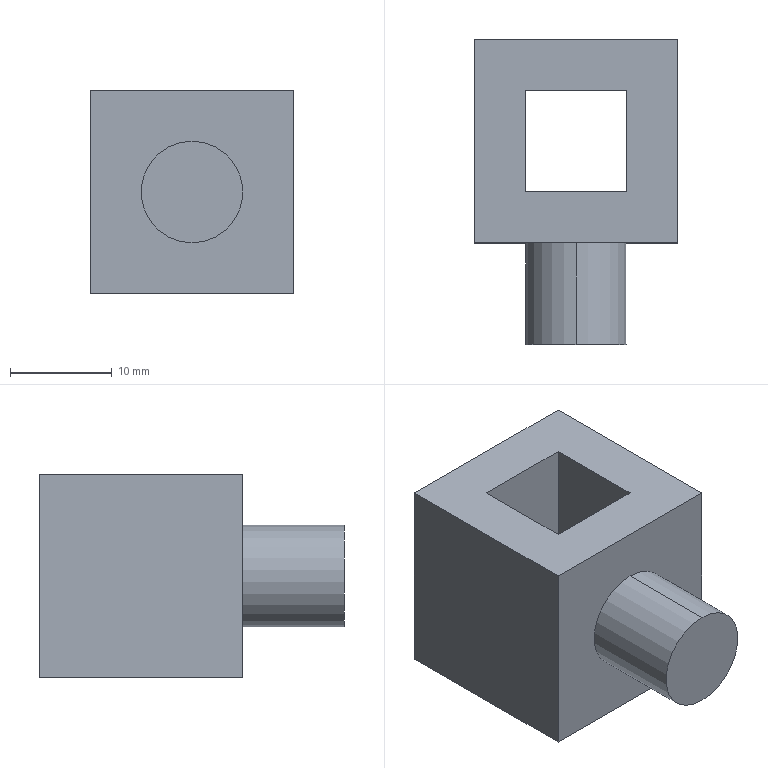Part | SolidWorks | features Extrusion 1, ICE 1 | 1 solid | 13 faces | box 20 x 30 x 20 mm | volume 6785 mm3 | plane 11 | cylinder 2 | commonest cylinder face diameters 10 x2
STEP:
#1=CARTESIAN_POINT('',(5.,-15.,-5.));
#2=VERTEX_POINT('',#1);
#3=CARTESIAN_POINT('',(5.,-15.,5.));
#4=VERTEX_POINT('',#3);
#5=CARTESIAN_POINT('',(5.,-15.,0.));
#6=DIRECTION('',(0.,-1.,0.));
#7=DIRECTION('',(0.,0.,-1.));
#8=AXIS2_PLACEMENT_3D('',#5,#6,#7);
#9=CIRCLE('',#8,5.);
#10=EDGE_CURVE('',#2,#4,#9,.T.);
#11=ORIENTED_EDGE('',*,*,#10,.F.);
#12=CARTESIAN_POINT('',(5.,-5.,-5.));
#13=VERTEX_POINT('',#12);
#14=CARTESIAN_POINT('',(5.,-15.,-5.));
#15=DIRECTION('',(0.,1.,0.));
#16=VECTOR('',#15,1000.);
#17=LINE('',#14,#16);
#18=EDGE_CURVE('',#2,#13,#17,.T.);
#19=ORIENTED_EDGE('',*,*,#18,.T.);
#20=CARTESIAN_POINT('',(5.,-5.,5.));
#21=VERTEX_POINT('',#20);
#22=CARTESIAN_POINT('',(5.,-5.,0.));
#23=DIRECTION('',(0.,-1.,0.));
#24=DIRECTION('',(0.,0.,1.));
#25=AXIS2_PLACEMENT_3D('',#22,#23,#24);
#26=CIRCLE('',#25,5.);
#27=EDGE_CURVE('',#13,#21,#26,.T.);
#28=ORIENTED_EDGE('',*,*,#27,.T.);
#29=CARTESIAN_POINT('',(5.,-15.,5.));
#30=DIRECTION('',(0.,1.,0.));
#31=VECTOR('',#30,1000.);
#32=LINE('',#29,#31);
#33=EDGE_CURVE('',#4,#21,#32,.T.);
#34=ORIENTED_EDGE('',*,*,#33,.F.);
#35=EDGE_LOOP('',(#11,#19,#28,#34));
#36=FACE_OUTER_BOUND('',#35,.T.);
#37=CARTESIAN_POINT('',(5.,-15.,0.));
#38=DIRECTION('',(0.,1.,0.));
#39=DIRECTION('',(0.,0.,1.));
#40=AXIS2_PLACEMENT_3D('',#37,#38,#39);
#41=CYLINDRICAL_SURFACE('',#40,5.);
#42=ADVANCED_FACE('',(#36),#41,.T.);
#43=CARTESIAN_POINT('',(-5.,-5.,-10.));
#44=VERTEX_POINT('',#43);
#45=CARTESIAN_POINT('',(15.,-5.,-10.));
#46=VERTEX_POINT('',#45);
#47=CARTESIAN_POINT('',(-5.,-5.,-10.));
#48=DIRECTION('',(1.,0.,0.));
#49=VECTOR('',#48,1000.);
#50=LINE('',#47,#49);
#51=EDGE_CURVE('',#44,#46,#50,.T.);
#52=ORIENTED_EDGE('',*,*,#51,.T.);
#53=CARTESIAN_POINT('',(15.,-5.,10.));
#54=VERTEX_POINT('',#53);
#55=CARTESIAN_POINT('',(15.,-5.,10.));
#56=DIRECTION('',(0.,0.,-1.));
#57=VECTOR('',#56,1000.);
#58=LINE('',#55,#57);
#59=EDGE_CURVE('',#54,#46,#58,.T.);
#60=ORIENTED_EDGE('',*,*,#59,.F.);
#61=CARTESIAN_POINT('',(-5.,-5.,10.));
#62=VERTEX_POINT('',#61);
#63=CARTESIAN_POINT('',(-5.,-5.,10.));
#64=DIRECTION('',(1.,0.,0.));
#65=VECTOR('',#64,1000.);
#66=LINE('',#63,#65);
#67=EDGE_CURVE('',#62,#54,#66,.T.);
#68=ORIENTED_EDGE('',*,*,#67,.F.);
#69=CARTESIAN_POINT('',(-5.,-5.,10.));
#70=DIRECTION('',(0.,0.,-1.));
#71=VECTOR('',#70,1000.);
#72=LINE('',#69,#71);
#73=EDGE_CURVE('',#62,#44,#72,.T.);
#74=ORIENTED_EDGE('',*,*,#73,.T.);
#75=EDGE_LOOP('',(#52,#60,#68,#74));
#76=FACE_OUTER_BOUND('',#75,.T.);
#77=CARTESIAN_POINT('',(5.,-5.,0.));
#78=DIRECTION('',(0.,-1.,0.));
#79=DIRECTION('',(0.,0.,1.));
#80=AXIS2_PLACEMENT_3D('',#77,#78,#79);
#81=CIRCLE('',#80,5.);
#82=EDGE_CURVE('',#21,#13,#81,.T.);
#83=ORIENTED_EDGE('',*,*,#82,.F.);
#84=ORIENTED_EDGE('',*,*,#27,.F.);
#85=EDGE_LOOP('',(#83,#84));
#86=FACE_BOUND('',#85,.T.);
#87=CARTESIAN_POINT('',(-5.,-5.,10.));
#88=DIRECTION('',(0.,1.,0.));
#89=DIRECTION('',(0.,0.,1.));
#90=AXIS2_PLACEMENT_3D('',#87,#88,#89);
#91=PLANE('',#90);
#92=ADVANCED_FACE('',(#76,#86),#91,.F.);
#93=CARTESIAN_POINT('',(-5.,15.,10.));
#94=VERTEX_POINT('',#93);
#95=CARTESIAN_POINT('',(-5.,-5.,10.));
#96=DIRECTION('',(0.,-1.,0.));
#97=VECTOR('',#96,1000.);
#98=LINE('',#95,#97);
#99=EDGE_CURVE('',#94,#62,#98,.T.);
#100=ORIENTED_EDGE('',*,*,#99,.T.);
#101=ORIENTED_EDGE('',*,*,#67,.T.);
#102=CARTESIAN_POINT('',(15.,15.,10.));
#103=VERTEX_POINT('',#102);
#104=CARTESIAN_POINT('',(15.,-5.,10.));
#105=DIRECTION('',(0.,1.,0.));
#106=VECTOR('',#105,1000.);
#107=LINE('',#104,#106);
#108=EDGE_CURVE('',#54,#103,#107,.T.);
#109=ORIENTED_EDGE('',*,*,#108,.T.);
#110=CARTESIAN_POINT('',(-5.,15.,10.));
#111=DIRECTION('',(-1.,0.,0.));
#112=VECTOR('',#111,1000.);
#113=LINE('',#110,#112);
#114=EDGE_CURVE('',#103,#94,#113,.T.);
#115=ORIENTED_EDGE('',*,*,#114,.T.);
#116=EDGE_LOOP('',(#100,#101,#109,#115));
#117=FACE_OUTER_BOUND('',#116,.T.);
#118=CARTESIAN_POINT('',(0.,10.,10.));
#119=VERTEX_POINT('',#118);
#120=CARTESIAN_POINT('',(0.,0.,10.));
#121=VERTEX_POINT('',#120);
#122=CARTESIAN_POINT('',(0.,0.,10.));
#123=DIRECTION('',(0.,-1.,0.));
#124=VECTOR('',#123,1000.);
#125=LINE('',#122,#124);
#126=EDGE_CURVE('',#119,#121,#125,.T.);
#127=ORIENTED_EDGE('',*,*,#126,.F.);
#128=CARTESIAN_POINT('',(10.,10.,10.));
#129=VERTEX_POINT('',#128);
#130=CARTESIAN_POINT('',(0.,10.,10.));
#131=DIRECTION('',(-1.,0.,0.));
#132=VECTOR('',#131,1000.);
#133=LINE('',#130,#132);
#134=EDGE_CURVE('',#129,#119,#133,.T.);
#135=ORIENTED_EDGE('',*,*,#134,.F.);
#136=CARTESIAN_POINT('',(10.,0.,10.));
#137=VERTEX_POINT('',#136);
#138=CARTESIAN_POINT('',(10.,0.,10.));
#139=DIRECTION('',(0.,1.,0.));
#140=VECTOR('',#139,1000.);
#141=LINE('',#138,#140);
#142=EDGE_CURVE('',#137,#129,#141,.T.);
#143=ORIENTED_EDGE('',*,*,#142,.F.);
#144=CARTESIAN_POINT('',(0.,0.,10.));
#145=DIRECTION('',(1.,0.,0.));
#146=VECTOR('',#145,1000.);
#147=LINE('',#144,#146);
#148=EDGE_CURVE('',#121,#137,#147,.T.);
#149=ORIENTED_EDGE('',*,*,#148,.F.);
#150=EDGE_LOOP('',(#127,#135,#143,#149));
#151=FACE_BOUND('',#150,.T.);
#152=CARTESIAN_POINT('',(0.,0.,10.));
#153=DIRECTION('',(0.,0.,-1.));
#154=DIRECTION('',(-1.,0.,0.));
#155=AXIS2_PLACEMENT_3D('',#152,#153,#154);
#156=PLANE('',#155);
#157=ADVANCED_FACE('',(#117,#151),#156,.F.);
#158=CARTESIAN_POINT('',(-5.,15.,-10.));
#159=VERTEX_POINT('',#158);
#160=CARTESIAN_POINT('',(-5.,-5.,-10.));
#161=DIRECTION('',(0.,-1.,0.));
#162=VECTOR('',#161,1000.);
#163=LINE('',#160,#162);
#164=EDGE_CURVE('',#159,#44,#163,.T.);
#165=ORIENTED_EDGE('',*,*,#164,.F.);
#166=CARTESIAN_POINT('',(15.,15.,-10.));
#167=VERTEX_POINT('',#166);
#168=CARTESIAN_POINT('',(-5.,15.,-10.));
#169=DIRECTION('',(-1.,0.,0.));
#170=VECTOR('',#169,1000.);
#171=LINE('',#168,#170);
#172=EDGE_CURVE('',#167,#159,#171,.T.);
#173=ORIENTED_EDGE('',*,*,#172,.F.);
#174=CARTESIAN_POINT('',(15.,-5.,-10.));
#175=DIRECTION('',(0.,1.,0.));
#176=VECTOR('',#175,1000.);
#177=LINE('',#174,#176);
#178=EDGE_CURVE('',#46,#167,#177,.T.);
#179=ORIENTED_EDGE('',*,*,#178,.F.);
#180=ORIENTED_EDGE('',*,*,#51,.F.);
#181=EDGE_LOOP('',(#165,#173,#179,#180));
#182=FACE_OUTER_BOUND('',#181,.T.);
#183=CARTESIAN_POINT('',(10.,10.,-10.));
#184=VERTEX_POINT('',#183);
#185=CARTESIAN_POINT('',(0.,10.,-10.));
#186=VERTEX_POINT('',#185);
#187=CARTESIAN_POINT('',(0.,10.,-10.));
#188=DIRECTION('',(-1.,0.,0.));
#189=VECTOR('',#188,1000.);
#190=LINE('',#187,#189);
#191=EDGE_CURVE('',#184,#186,#190,.T.);
#192=ORIENTED_EDGE('',*,*,#191,.T.);
#193=CARTESIAN_POINT('',(0.,0.,-10.));
#194=VERTEX_POINT('',#193);
#195=CARTESIAN_POINT('',(0.,0.,-10.));
#196=DIRECTION('',(0.,-1.,0.));
#197=VECTOR('',#196,1000.);
#198=LINE('',#195,#197);
#199=EDGE_CURVE('',#186,#194,#198,.T.);
#200=ORIENTED_EDGE('',*,*,#199,.T.);
#201=CARTESIAN_POINT('',(10.,0.,-10.));
#202=VERTEX_POINT('',#201);
#203=CARTESIAN_POINT('',(0.,0.,-10.));
#204=DIRECTION('',(1.,0.,0.));
#205=VECTOR('',#204,1000.);
#206=LINE('',#203,#205);
#207=EDGE_CURVE('',#194,#202,#206,.T.);
#208=ORIENTED_EDGE('',*,*,#207,.T.);
#209=CARTESIAN_POINT('',(10.,0.,-10.));
#210=DIRECTION('',(0.,1.,0.));
#211=VECTOR('',#210,1000.);
#212=LINE('',#209,#211);
#213=EDGE_CURVE('',#202,#184,#212,.T.);
#214=ORIENTED_EDGE('',*,*,#213,.T.);
#215=EDGE_LOOP('',(#192,#200,#208,#214));
#216=FACE_BOUND('',#215,.T.);
#217=CARTESIAN_POINT('',(0.,0.,-10.));
#218=DIRECTION('',(0.,0.,-1.));
#219=DIRECTION('',(-1.,0.,0.));
#220=AXIS2_PLACEMENT_3D('',#217,#218,#219);
#221=PLANE('',#220);
#222=ADVANCED_FACE('',(#182,#216),#221,.T.);
#223=ORIENTED_EDGE('',*,*,#164,.T.);
#224=ORIENTED_EDGE('',*,*,#73,.F.);
#225=ORIENTED_EDGE('',*,*,#99,.F.);
#226=CARTESIAN_POINT('',(-5.,15.,10.));
#227=DIRECTION('',(0.,0.,-1.));
#228=VECTOR('',#227,1000.);
#229=LINE('',#226,#228);
#230=EDGE_CURVE('',#94,#159,#229,.T.);
#231=ORIENTED_EDGE('',*,*,#230,.T.);
#232=EDGE_LOOP('',(#223,#224,#225,#231));
#233=FACE_OUTER_BOUND('',#232,.T.);
#234=CARTESIAN_POINT('',(-5.,-5.,10.));
#235=DIRECTION('',(1.,0.,0.));
#236=DIRECTION('',(0.,0.,-1.));
#237=AXIS2_PLACEMENT_3D('',#234,#235,#236);
#238=PLANE('',#237);
#239=ADVANCED_FACE('',(#233),#238,.F.);
#240=ORIENTED_EDGE('',*,*,#178,.T.);
#241=CARTESIAN_POINT('',(15.,15.,10.));
#242=DIRECTION('',(0.,0.,-1.));
#243=VECTOR('',#242,1000.);
#244=LINE('',#241,#243);
#245=EDGE_CURVE('',#103,#167,#244,.T.);
#246=ORIENTED_EDGE('',*,*,#245,.F.);
#247=ORIENTED_EDGE('',*,*,#108,.F.);
#248=ORIENTED_EDGE('',*,*,#59,.T.);
#249=EDGE_LOOP('',(#240,#246,#247,#248));
#250=FACE_OUTER_BOUND('',#249,.T.);
#251=CARTESIAN_POINT('',(15.,-5.,10.));
#252=DIRECTION('',(-1.,0.,0.));
#253=DIRECTION('',(0.,0.,1.));
#254=AXIS2_PLACEMENT_3D('',#251,#252,#253);
#255=PLANE('',#254);
#256=ADVANCED_FACE('',(#250),#255,.F.);
#257=ORIENTED_EDGE('',*,*,#172,.T.);
#258=ORIENTED_EDGE('',*,*,#230,.F.);
#259=ORIENTED_EDGE('',*,*,#114,.F.);
#260=ORIENTED_EDGE('',*,*,#245,.T.);
#261=EDGE_LOOP('',(#257,#258,#259,#260));
#262=FACE_OUTER_BOUND('',#261,.T.);
#263=CARTESIAN_POINT('',(-5.,15.,10.));
#264=DIRECTION('',(0.,-1.,0.));
#265=DIRECTION('',(0.,0.,-1.));
#266=AXIS2_PLACEMENT_3D('',#263,#264,#265);
#267=PLANE('',#266);
#268=ADVANCED_FACE('',(#262),#267,.F.);
#269=ORIENTED_EDGE('',*,*,#199,.F.);
#270=CARTESIAN_POINT('',(0.,10.,10.));
#271=DIRECTION('',(0.,0.,-1.));
#272=VECTOR('',#271,1000.);
#273=LINE('',#270,#272);
#274=EDGE_CURVE('',#119,#186,#273,.T.);
#275=ORIENTED_EDGE('',*,*,#274,.F.);
#276=ORIENTED_EDGE('',*,*,#126,.T.);
#277=CARTESIAN_POINT('',(0.,0.,10.));
#278=DIRECTION('',(0.,0.,-1.));
#279=VECTOR('',#278,1000.);
#280=LINE('',#277,#279);
#281=EDGE_CURVE('',#121,#194,#280,.T.);
#282=ORIENTED_EDGE('',*,*,#281,.T.);
#283=EDGE_LOOP('',(#269,#275,#276,#282));
#284=FACE_OUTER_BOUND('',#283,.T.);
#285=CARTESIAN_POINT('',(0.,0.,10.));
#286=DIRECTION('',(1.,0.,0.));
#287=DIRECTION('',(0.,0.,-1.));
#288=AXIS2_PLACEMENT_3D('',#285,#286,#287);
#289=PLANE('',#288);
#290=ADVANCED_FACE('',(#284),#289,.T.);
#291=ORIENTED_EDGE('',*,*,#207,.F.);
#292=ORIENTED_EDGE('',*,*,#281,.F.);
#293=ORIENTED_EDGE('',*,*,#148,.T.);
#294=CARTESIAN_POINT('',(10.,0.,10.));
#295=DIRECTION('',(0.,0.,-1.));
#296=VECTOR('',#295,1000.);
#297=LINE('',#294,#296);
#298=EDGE_CURVE('',#137,#202,#297,.T.);
#299=ORIENTED_EDGE('',*,*,#298,.T.);
#300=EDGE_LOOP('',(#291,#292,#293,#299));
#301=FACE_OUTER_BOUND('',#300,.T.);
#302=CARTESIAN_POINT('',(0.,0.,10.));
#303=DIRECTION('',(0.,1.,0.));
#304=DIRECTION('',(0.,0.,1.));
#305=AXIS2_PLACEMENT_3D('',#302,#303,#304);
#306=PLANE('',#305);
#307=ADVANCED_FACE('',(#301),#306,.T.);
#308=ORIENTED_EDGE('',*,*,#213,.F.);
#309=ORIENTED_EDGE('',*,*,#298,.F.);
#310=ORIENTED_EDGE('',*,*,#142,.T.);
#311=CARTESIAN_POINT('',(10.,10.,10.));
#312=DIRECTION('',(0.,0.,-1.));
#313=VECTOR('',#312,1000.);
#314=LINE('',#311,#313);
#315=EDGE_CURVE('',#129,#184,#314,.T.);
#316=ORIENTED_EDGE('',*,*,#315,.T.);
#317=EDGE_LOOP('',(#308,#309,#310,#316));
#318=FACE_OUTER_BOUND('',#317,.T.);
#319=CARTESIAN_POINT('',(10.,0.,10.));
#320=DIRECTION('',(-1.,0.,0.));
#321=DIRECTION('',(0.,0.,1.));
#322=AXIS2_PLACEMENT_3D('',#319,#320,#321);
#323=PLANE('',#322);
#324=ADVANCED_FACE('',(#318),#323,.T.);
#325=ORIENTED_EDGE('',*,*,#191,.F.);
#326=ORIENTED_EDGE('',*,*,#315,.F.);
#327=ORIENTED_EDGE('',*,*,#134,.T.);
#328=ORIENTED_EDGE('',*,*,#274,.T.);
#329=EDGE_LOOP('',(#325,#326,#327,#328));
#330=FACE_OUTER_BOUND('',#329,.T.);
#331=CARTESIAN_POINT('',(0.,10.,10.));
#332=DIRECTION('',(0.,-1.,0.));
#333=DIRECTION('',(1.,0.,0.));
#334=AXIS2_PLACEMENT_3D('',#331,#332,#333);
#335=PLANE('',#334);
#336=ADVANCED_FACE('',(#330),#335,.T.);
#337=ORIENTED_EDGE('',*,*,#18,.F.);
#338=CARTESIAN_POINT('',(5.,-15.,0.));
#339=DIRECTION('',(0.,-1.,0.));
#340=DIRECTION('',(0.,0.,-1.));
#341=AXIS2_PLACEMENT_3D('',#338,#339,#340);
#342=CIRCLE('',#341,5.);
#343=EDGE_CURVE('',#4,#2,#342,.T.);
#344=ORIENTED_EDGE('',*,*,#343,.F.);
#345=ORIENTED_EDGE('',*,*,#33,.T.);
#346=ORIENTED_EDGE('',*,*,#82,.T.);
#347=EDGE_LOOP('',(#337,#344,#345,#346));
#348=FACE_OUTER_BOUND('',#347,.T.);
#349=CARTESIAN_POINT('',(5.,-15.,0.));
#350=DIRECTION('',(0.,1.,0.));
#351=DIRECTION('',(0.,0.,1.));
#352=AXIS2_PLACEMENT_3D('',#349,#350,#351);
#353=CYLINDRICAL_SURFACE('',#352,5.);
#354=ADVANCED_FACE('',(#348),#353,.T.);
#355=ORIENTED_EDGE('',*,*,#343,.T.);
#356=ORIENTED_EDGE('',*,*,#10,.T.);
#357=EDGE_LOOP('',(#355,#356));
#358=FACE_OUTER_BOUND('',#357,.T.);
#359=CARTESIAN_POINT('',(5.,-15.,0.));
#360=DIRECTION('',(0.,-1.,0.));
#361=DIRECTION('',(0.,0.,-1.));
#362=AXIS2_PLACEMENT_3D('',#359,#360,#361);
#363=PLANE('',#362);
#364=ADVANCED_FACE('',(#358),#363,.T.);
#365=CLOSED_SHELL('',(#42,#92,#157,#222,#239,#256,#268,#290,#307,#324,#336,#354,#364));
#366=MANIFOLD_SOLID_BREP('',#365);
#367=CARTESIAN_POINT('',(0.,0.,0.));
#368=DIRECTION('',(0.,0.,1.));
#369=DIRECTION('',(1.,0.,0.));
#370=AXIS2_PLACEMENT_3D('',#367,#368,#369);
#371=(LENGTH_UNIT()NAMED_UNIT(*)SI_UNIT(.MILLI.,.METRE.));
#372=UNCERTAINTY_MEASURE_WITH_UNIT(LENGTH_MEASURE(0.00001),#371,'','');
#373=(NAMED_UNIT(*)PLANE_ANGLE_UNIT()SI_UNIT($,.RADIAN.));
#374=(NAMED_UNIT(*)SI_UNIT($,.STERADIAN.)SOLID_ANGLE_UNIT());
#375=(GEOMETRIC_REPRESENTATION_CONTEXT(3)GLOBAL_UNCERTAINTY_ASSIGNED_CONTEXT((#372))GLOBAL_UNIT_ASSIGNED_CONTEXT((#371,#373,#374))REPRESENTATION_CONTEXT('',''));
#376=ADVANCED_BREP_SHAPE_REPRESENTATION('',(#366,#370),#375);